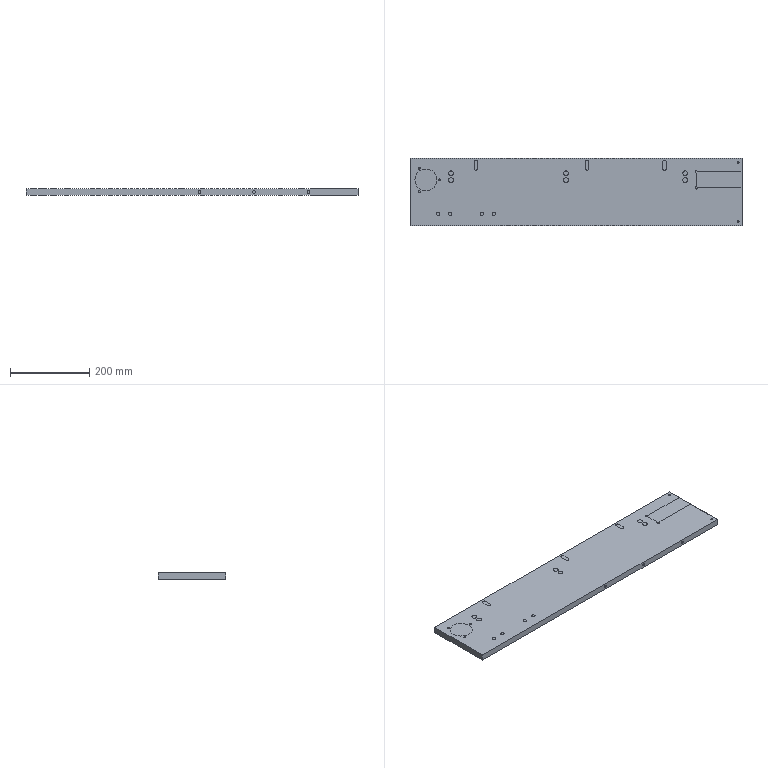NC program | NX | posted with a generic post | part box 836 x 170 x 16 mm
Lines 8598 to 9504 of 11551:
(等高清角 , TOOL : D4平底刀)
N17176 T16 M6
N17178 /M1
N17180 G17 G43 G0 G90 X721.292 Y95.484 Z100. S3000 H16 M3
N17182 Z0.1
N17184 G94 G1 Z-0.1 F800.
N17186 G3 X720.926 Y96.246 R0.45
N17188 X721.75 Y95.5 R-0.75 F1000.
N17190 G2 X721.97 Y96.47 R2.25
N17192 X721. Y96.25 R2.25
N17194 G1 X720.926 Y96.246
N17196 G3 X720.717 Y95.427 R0.45
N17198 G1 Z0.1
N17200 G0 Z0.
N17202 G1 Z-0.2 F800.
N17204 G2 X720.926 Y96.246 R0.45
N17206 G1 X721. Y96.25 F1000.
N17208 G3 X721.97 Y96.47 R2.25
N17210 X721.75 Y95.5 R2.25
N17212 G2 X720.926 Y96.246 R-0.75
N17214 X721.292 Y95.484 R0.45
N17216 G1 Z0.
N17218 G0 Z-0.1
N17220 G1 Z-0.3 F800.
N17222 G3 X720.926 Y96.246 R0.45
N17224 X721.75 Y95.5 R-0.75 F1000.
N17226 G2 X721.97 Y96.47 R2.25
N17228 X721. Y96.25 R2.25
N17230 G1 X720.926 Y96.246
N17232 G3 X720.717 Y95.427 R0.45
N17234 G1 Z-0.1
N17236 G0 Z-0.2
N17238 G1 Z-0.4 F800.
N17240 G2 X720.926 Y96.246 R0.45
N17242 G1 X721. Y96.25 F1000.
N17244 G3 X721.97 Y96.47 R2.25
N17246 X721.75 Y95.5 R2.25
N17248 G2 X720.926 Y96.246 R-0.75
N17250 X721.292 Y95.484 R0.45
N17252 G1 Z-0.2
N17254 G0 Z-0.3
N17256 G1 Z-0.5 F800.
N17258 G3 X720.926 Y96.246 R0.45
N17260 X721.75 Y95.5 R-0.75 F1000.
N17262 G2 X721.97 Y96.47 R2.25
N17264 X721. Y96.25 R2.25
N17266 G1 X720.926 Y96.246
N17268 G3 X720.717 Y95.427 R0.45
N17270 G1 Z-0.3
N17272 G0 Z-0.4
N17274 G1 Z-0.6 F800.
N17276 G2 X720.926 Y96.246 R0.45
N17278 G1 X721. Y96.25 F1000.
N17280 G3 X721.97 Y96.47 R2.25
N17282 X721.75 Y95.5 R2.25
N17284 G2 X720.926 Y96.246 R-0.75
N17286 X721.292 Y95.484 R0.45
N17288 G1 Z-0.4
N17290 G0 Z-0.5
N17292 G1 Z-0.7 F800.
N17294 G3 X720.926 Y96.246 R0.45
N17296 X721.75 Y95.5 R-0.75 F1000.
N17298 G2 X721.97 Y96.47 R2.25
N17300 X721. Y96.25 R2.25
N17302 G1 X720.926 Y96.246
N17304 G3 X720.717 Y95.427 R0.45
N17306 G1 Z-0.5
N17308 G0 Z-0.6
N17310 G1 Z-0.8 F800.
N17312 G2 X720.926 Y96.246 R0.45
N17314 G1 X721. Y96.25 F1000.
N17316 G3 X721.97 Y96.47 R2.25
N17318 X721.75 Y95.5 R2.25
N17320 G2 X720.926 Y96.246 R-0.75
N17322 X721.292 Y95.484 R0.45
N17324 G1 Z-0.6
N17326 G0 Z-0.7
N17328 G1 Z-0.9 F800.
N17330 G3 X720.926 Y96.246 R0.45
N17332 X721.75 Y95.5 R-0.75 F1000.
N17334 G2 X721.97 Y96.47 R2.25
N17336 X721. Y96.25 R2.25
N17338 G1 X720.926 Y96.246
N17340 G3 X720.717 Y95.427 R0.45
N17342 G1 Z-0.7
N17344 G0 Z-0.8
N17346 G1 Z-1. F800.
N17348 G2 X720.926 Y96.246 R0.45
N17350 G1 X721. Y96.25 F1000.
N17352 G3 X721.97 Y96.47 R2.25
N17354 X721.75 Y95.5 R2.25
N17356 G2 X720.926 Y96.246 R-0.75
N17358 X721.292 Y95.484 R0.45
N17360 G1 Z-0.8
N17362 G0 Z-0.9
N17364 G1 Z-1.1 F800.
N17366 G3 X720.926 Y96.246 R0.45
N17368 X721.75 Y95.5 R-0.75 F1000.
N17370 G2 X721.97 Y96.47 R2.25
N17372 X721. Y96.25 R2.25
N17374 G1 X720.926 Y96.246
N17376 G3 X720.717 Y95.427 R0.45
N17378 G1 Z-0.9
N17380 G0 Z-1.
N17382 G1 Z-1.2 F800.
N17384 G2 X720.926 Y96.246 R0.45
N17386 G1 X721. Y96.25 F1000.
N17388 G3 X721.97 Y96.47 R2.25
N17390 X721.75 Y95.5 R2.25
N17392 G2 X720.926 Y96.246 R-0.75
N17394 X721.292 Y95.484 R0.45
N17396 G1 Z-1.
N17398 G0 Z-1.1
N17400 G1 Z-1.3 F800.
N17402 G3 X720.926 Y96.246 R0.45
N17404 X721.75 Y95.5 R-0.75 F1000.
N17406 G2 X721.97 Y96.47 R2.25
N17408 X721. Y96.25 R2.25
N17410 G1 X720.926 Y96.246
N17412 G3 X720.717 Y95.427 R0.45
N17414 G1 Z-1.1
N17416 G0 Z-1.2
N17418 G1 Z-1.4 F800.
N17420 G2 X720.926 Y96.246 R0.45
N17422 G1 X721. Y96.25 F1000.
N17424 G3 X721.97 Y96.47 R2.25
N17426 X721.75 Y95.5 R2.25
N17428 G2 X720.926 Y96.246 R-0.75
N17430 X721.292 Y95.484 R0.45
N17432 G1 Z-1.2
N17434 G0 Z-1.3
N17436 G1 Z-1.5 F800.
N17438 G3 X720.926 Y96.246 R0.45
N17440 X721.75 Y95.5 R-0.75 F1000.
N17442 G2 X721.97 Y96.47 R2.25
N17444 X721. Y96.25 R2.25
N17446 G1 X720.926 Y96.246
N17448 G3 X720.717 Y95.427 R0.45
N17450 G1 Z-1.3
N17452 G0 Z-1.4
N17454 G1 Z-1.6 F800.
N17456 G2 X720.926 Y96.246 R0.45
N17458 G1 X721. Y96.25 F1000.
N17460 G3 X721.97 Y96.47 R2.25
N17462 X721.75 Y95.5 R2.25
N17464 G2 X720.926 Y96.246 R-0.75
N17466 X721.292 Y95.484 R0.45
N17468 G1 Z-1.4
N17470 G0 Z-1.5
N17472 G1 Z-1.7 F800.
N17474 G3 X720.926 Y96.246 R0.45
N17476 X721.75 Y95.5 R-0.75 F1000.
N17478 G2 X721.97 Y96.47 R2.25
N17480 X721. Y96.25 R2.25
N17482 G1 X720.926 Y96.246
N17484 G3 X720.717 Y95.427 R0.45
N17486 G1 Z-1.5
N17488 G0 Z-1.6
N17490 G1 Z-1.8 F800.
N17492 G2 X720.926 Y96.246 R0.45
N17494 G1 X721. Y96.25 F1000.
N17496 G3 X721.97 Y96.47 R2.25
N17498 X721.75 Y95.5 R2.25
N17500 G2 X720.926 Y96.246 R-0.75
N17502 X721.292 Y95.484 R0.45
N17504 G1 Z-1.6
N17506 G0 Z-1.7
N17508 G1 Z-1.9 F800.
N17510 G3 X720.926 Y96.246 R0.45
N17512 X721.75 Y95.5 R-0.75 F1000.
N17514 G2 X721.97 Y96.47 R2.25
N17516 X721. Y96.25 R2.25
N17518 G1 X720.926 Y96.246
N17520 G3 X720.717 Y95.427 R0.45
N17522 G1 Z-1.7
N17524 G0 Z-1.8
N17526 G1 Z-2. F800.
N17528 G2 X720.926 Y96.246 R0.45
N17530 G1 X721. Y96.25 F1000.
N17532 G3 X721.97 Y96.47 R2.25
N17534 X721.75 Y95.5 R2.25
N17536 G2 X720.926 Y96.246 R-0.75
N17538 X721.292 Y95.484 R0.45
N17540 G1 Z-1.8
N17542 G0 Z-1.9
N17544 G1 Z-2.1 F800.
N17546 G3 X720.926 Y96.246 R0.45
N17548 X721.75 Y95.5 R-0.75 F1000.
N17550 G2 X721.97 Y96.47 R2.25
N17552 X721. Y96.25 R2.25
N17554 G1 X720.926 Y96.246
N17556 G3 X720.717 Y95.427 R0.45
N17558 G1 Z-1.9
N17560 G0 Z-2.
N17562 G1 Z-2.2 F800.
N17564 G2 X720.926 Y96.246 R0.45
N17566 G1 X721. Y96.25 F1000.
N17568 G3 X721.97 Y96.47 R2.25
N17570 X721.75 Y95.5 R2.25
N17572 G2 X720.926 Y96.246 R-0.75
N17574 X721.292 Y95.484 R0.45
N17576 G1 Z-2.
N17578 G0 Z-2.1
N17580 G1 Z-2.3 F800.
N17582 G3 X720.926 Y96.246 R0.45
N17584 X721.75 Y95.5 R-0.75 F1000.
N17586 G2 X721.97 Y96.47 R2.25
N17588 X721. Y96.25 R2.25
N17590 G1 X720.926 Y96.246
N17592 G3 X720.717 Y95.427 R0.45
N17594 G1 Z-2.1
N17596 G0 Z-2.2
N17598 G1 Z-2.4 F800.
N17600 G2 X720.926 Y96.246 R0.45
N17602 G1 X721. Y96.25 F1000.
N17604 G3 X721.97 Y96.47 R2.25
N17606 X721.75 Y95.5 R2.25
N17608 G2 X720.926 Y96.246 R-0.75
N17610 X721.292 Y95.484 R0.45
N17612 G1 Z-2.2
N17614 G0 Z-2.3
N17616 G1 Z-2.5 F800.
N17618 G3 X720.926 Y96.246 R0.45
N17620 X721.75 Y95.5 R-0.75 F1000.
N17622 G2 X721.97 Y96.47 R2.25
N17624 X721. Y96.25 R2.25
N17626 G1 X720.926 Y96.246
N17628 G3 X720.717 Y95.427 R0.45
N17630 G1 Z-2.3
N17632 G0 Z-2.4
N17634 G1 Z-2.6 F800.
N17636 G2 X720.926 Y96.246 R0.45
N17638 G1 X721. Y96.25 F1000.
N17640 G3 X721.97 Y96.47 R2.25
N17642 X721.75 Y95.5 R2.25
N17644 G2 X720.926 Y96.246 R-0.75
N17646 X721.292 Y95.484 R0.45
N17648 G1 Z-2.4
N17650 G0 Z-2.5
N17652 G1 Z-2.7 F800.
N17654 G3 X720.926 Y96.246 R0.45
N17656 X721.75 Y95.5 R-0.75 F1000.
N17658 G2 X721.97 Y96.47 R2.25
N17660 X721. Y96.25 R2.25
N17662 G1 X720.926 Y96.246
N17664 G3 X720.717 Y95.427 R0.45
N17666 G1 Z-2.5
N17668 G0 Z-2.6
N17670 G1 Z-2.8 F800.
N17672 G2 X720.926 Y96.246 R0.45
N17674 G1 X721. Y96.25 F1000.
N17676 G3 X721.97 Y96.47 R2.25
N17678 X721.75 Y95.5 R2.25
N17680 G2 X720.926 Y96.246 R-0.75
N17682 X721.292 Y95.484 R0.45
N17684 G1 Z-2.6
N17686 G0 Z-2.7
N17688 G1 Z-2.9 F800.
N17690 G3 X720.926 Y96.246 R0.45
N17692 X721.75 Y95.5 R-0.75 F1000.
N17694 G2 X721.97 Y96.47 R2.25
N17696 X721. Y96.25 R2.25
N17698 G1 X720.926 Y96.246
N17700 G3 X720.717 Y95.427 R0.45
N17702 G1 Z-2.7
N17704 G0 Z-2.8
N17706 G1 Z-3. F800.
N17708 G2 X720.926 Y96.246 R0.45
N17710 G1 X721. Y96.25 F1000.
N17712 G3 X721.97 Y96.47 R2.25
N17714 X721.75 Y95.5 R2.25
N17716 G2 X720.926 Y96.246 R-0.75
N17718 X721.292 Y95.484 R0.45
N17720 G1 Z-2.8
N17722 G0 Z-2.9
N17724 G1 Z-3.1 F800.
N17726 G3 X720.926 Y96.246 R0.45
N17728 X721.75 Y95.5 R-0.75 F1000.
N17730 G2 X721.97 Y96.47 R2.25
N17732 X721. Y96.25 R2.25
N17734 G1 X720.926 Y96.246
N17736 G3 X720.717 Y95.427 R0.45
N17738 G1 Z-2.9
N17740 G0 Z-3.
N17742 G1 Z-3.2 F800.
N17744 G2 X720.926 Y96.246 R0.45
N17746 G1 X721. Y96.25 F1000.
N17748 G3 X721.97 Y96.47 R2.25
N17750 X721.75 Y95.5 R2.25
N17752 G2 X720.926 Y96.246 R-0.75
N17754 X721.292 Y95.484 R0.45
N17756 G1 Z-3.
N17758 G0 Z-3.1
N17760 G1 Z-3.3 F800.
N17762 G3 X720.926 Y96.246 R0.45
N17764 X721.75 Y95.5 R-0.75 F1000.
N17766 G2 X721.97 Y96.47 R2.25
N17768 X721. Y96.25 R2.25
N17770 G1 X720.926 Y96.246
N17772 G3 X720.717 Y95.427 R0.45
N17774 G1 Z-3.1
N17776 G0 Z-3.2
N17778 G1 Z-3.4 F800.
N17780 G2 X720.926 Y96.246 R0.45
N17782 G1 X721. Y96.25 F1000.
N17784 G3 X721.97 Y96.47 R2.25
N17786 X721.75 Y95.5 R2.25
N17788 G2 X720.926 Y96.246 R-0.75
N17790 X721.292 Y95.484 R0.45
N17792 G1 Z-3.2
N17794 G0 Z-3.3
N17796 G1 Z-3.5 F800.
N17798 G3 X720.926 Y96.246 R0.45
N17800 X721.75 Y95.5 R-0.75 F1000.
N17802 G2 X721.97 Y96.47 R2.25
N17804 X721. Y96.25 R2.25
N17806 G1 X720.926 Y96.246
N17808 G3 X720.717 Y95.427 R0.45
N17810 G1 Z-3.3
N17812 G0 Z-3.4
N17814 G1 Z-3.6 F800.
N17816 G2 X720.926 Y96.246 R0.45
N17818 G1 X721. Y96.25 F1000.
N17820 G3 X721.97 Y96.47 R2.25
N17822 X721.75 Y95.5 R2.25
N17824 G2 X720.926 Y96.246 R-0.75
N17826 X721.292 Y95.484 R0.45
N17828 G1 Z-3.4
N17830 G0 Z-3.5
N17832 G1 Z-3.7 F800.
N17834 G3 X720.926 Y96.246 R0.45
N17836 X721.75 Y95.5 R-0.75 F1000.
N17838 G2 X721.97 Y96.47 R2.25
N17840 X721. Y96.25 R2.25
N17842 G1 X720.926 Y96.246
N17844 G3 X720.717 Y95.427 R0.45
N17846 G1 Z-3.5
N17848 G0 Z-3.6
N17850 G1 Z-3.8 F800.
N17852 G2 X720.926 Y96.246 R0.45
N17854 G1 X721. Y96.25 F1000.
N17856 G3 X721.97 Y96.47 R2.25
N17858 X721.75 Y95.5 R2.25
N17860 G2 X720.926 Y96.246 R-0.75
N17862 X721.292 Y95.484 R0.45
N17864 G1 Z-3.6
N17866 G0 Z-3.7
N17868 G1 Z-3.9 F800.
N17870 G3 X720.926 Y96.246 R0.45
N17872 X721.75 Y95.5 R-0.75 F1000.
N17874 G2 X721.97 Y96.47 R2.25
N17876 X721. Y96.25 R2.25
N17878 G1 X720.926 Y96.246
N17880 G3 X720.717 Y95.427 R0.45
N17882 G1 Z-3.7
N17884 G0 Z-3.8
N17886 G1 Z-4. F800.
N17888 G2 X720.926 Y96.246 R0.45
N17890 G1 X721. Y96.25 F1000.
N17892 G3 X721.97 Y96.47 R2.25
N17894 X721.75 Y95.5 R2.25
N17896 G2 X720.926 Y96.246 R-0.75
N17898 X721.292 Y95.484 R0.45
N17900 G1 Z-3.8
N17902 G0 Z-3.9
N17904 G1 Z-4.1 F800.
N17906 G3 X720.926 Y96.246 R0.45
N17908 X721.75 Y95.5 R-0.75 F1000.
N17910 G2 X721.97 Y96.47 R2.25
N17912 X721. Y96.25 R2.25
N17914 G1 X720.926 Y96.246
N17916 G3 X720.717 Y95.427 R0.45
N17918 G1 Z-3.9
N17920 G0 Z-4.
N17922 G1 Z-4.2 F800.
N17924 G2 X720.926 Y96.246 R0.45
N17926 G1 X721. Y96.25 F1000.
N17928 G3 X721.97 Y96.47 R2.25
N17930 X721.75 Y95.5 R2.25
N17932 G2 X720.926 Y96.246 R-0.75
N17934 X721.292 Y95.484 R0.45
N17936 G1 Z-4.
N17938 G0 Z-4.1
N17940 G1 Z-4.3 F800.
N17942 G3 X720.926 Y96.246 R0.45
N17944 X721.75 Y95.5 R-0.75 F1000.
N17946 G2 X721.97 Y96.47 R2.25
N17948 X721. Y96.25 R2.25
N17950 G1 X720.926 Y96.246
N17952 G3 X720.717 Y95.427 R0.45
N17954 G1 Z-4.1
N17956 G0 Z-4.2
N17958 G1 Z-4.4 F800.
N17960 G2 X720.926 Y96.246 R0.45
N17962 G1 X721. Y96.25 F1000.
N17964 G3 X721.97 Y96.47 R2.25
N17966 X721.75 Y95.5 R2.25
N17968 G2 X720.926 Y96.246 R-0.75
N17970 X721.292 Y95.484 R0.45
N17972 G1 Z-4.2
N17974 G0 Z-4.3
N17976 G1 Z-4.5 F800.
N17978 G3 X720.926 Y96.246 R0.45
N17980 X721.75 Y95.5 R-0.75 F1000.
N17982 G2 X721.97 Y96.47 R2.25
N17984 X721. Y96.25 R2.25
N17986 G1 X720.926 Y96.246
N17988 G3 X720.717 Y95.427 R0.45
N17990 G1 Z-4.3
N17992 G0 Z-4.4
N17994 G1 Z-4.6 F800.
N17996 G2 X720.926 Y96.246 R0.45
N17998 G1 X721. Y96.25 F1000.
N18000 G3 X721.97 Y96.47 R2.25
N18002 X721.75 Y95.5 R2.25
N18004 G2 X720.926 Y96.246 R-0.75
N18006 X721.292 Y95.484 R0.45
N18008 G1 Z-4.4
N18010 G0 Z-4.5
N18012 G1 Z-4.7 F800.
N18014 G3 X720.926 Y96.246 R0.45
N18016 X721.75 Y95.5 R-0.75 F1000.
N18018 G2 X721.97 Y96.47 R2.25
N18020 X721. Y96.25 R2.25
N18022 G1 X720.926 Y96.246
N18024 G3 X720.717 Y95.427 R0.45
N18026 G1 Z-4.5
N18028 G0 Z-4.6
N18030 G1 Z-4.8 F800.
N18032 G2 X720.926 Y96.246 R0.45
N18034 G1 X721. Y96.25 F1000.
N18036 G3 X721.97 Y96.47 R2.25
N18038 X721.75 Y95.5 R2.25
N18040 G2 X720.926 Y96.246 R-0.75
N18042 X721.292 Y95.484 R0.45
N18044 G1 Z-4.6
N18046 G0 Z-4.7
N18048 G1 Z-4.9 F800.
N18050 G3 X720.926 Y96.246 R0.45
N18052 X721.75 Y95.5 R-0.75 F1000.
N18054 G2 X721.97 Y96.47 R2.25
N18056 X721. Y96.25 R2.25
N18058 G1 X720.926 Y96.246
N18060 G3 X720.717 Y95.427 R0.45
N18062 G1 Z-4.7
N18064 G0 Z-4.8
N18066 G1 Z-5. F800.
N18068 G2 X720.926 Y96.246 R0.45
N18070 G1 X721. Y96.25 F1000.
N18072 G3 X721.97 Y96.47 R2.25
N18074 X721.75 Y95.5 R2.25
N18076 G2 X720.926 Y96.246 R-0.75
N18078 X721.292 Y95.484 R0.45
N18080 G1 Z-4.8
N18082 G0 Z-4.9
N18084 G1 Z-5.1 F800.
N18086 G3 X720.926 Y96.246 R0.45
N18088 X721.75 Y95.5 R-0.75 F1000.
N18090 G2 X721.97 Y96.47 R2.25
N18092 X721. Y96.25 R2.25
N18094 G1 X720.926 Y96.246
N18096 G3 X720.717 Y95.427 R0.45
N18098 G1 Z-4.9
N18100 G0 Z-5.
N18102 G1 Z-5.2 F800.
N18104 G2 X720.926 Y96.246 R0.45
N18106 G1 X721. Y96.25 F1000.
N18108 G3 X721.97 Y96.47 R2.25
N18110 X721.75 Y95.5 R2.25
N18112 G2 X720.926 Y96.246 R-0.75
N18114 X721.292 Y95.484 R0.45
N18116 G1 Z-5.
N18118 G0 Z-5.1
N18120 G1 Z-5.3 F800.
N18122 G3 X720.926 Y96.246 R0.45
N18124 X721.75 Y95.5 R-0.75 F1000.
N18126 G2 X721.97 Y96.47 R2.25
N18128 X721. Y96.25 R2.25
N18130 G1 X720.926 Y96.246
N18132 G3 X720.717 Y95.427 R0.45
N18134 G1 Z-5.1
N18136 G0 Z-5.2
N18138 G1 Z-5.4 F800.
N18140 G2 X720.926 Y96.246 R0.45
N18142 G1 X721. Y96.25 F1000.
N18144 G3 X721.97 Y96.47 R2.25
N18146 X721.75 Y95.5 R2.25
N18148 G2 X720.926 Y96.246 R-0.75
N18150 X721.292 Y95.484 R0.45
N18152 G1 Z-5.2
N18154 G0 Z-5.3
N18156 G1 Z-5.5 F800.
N18158 G3 X720.926 Y96.246 R0.45
N18160 X721.75 Y95.5 R-0.75 F1000.
N18162 G2 X721.97 Y96.47 R2.25
N18164 X721. Y96.25 R2.25
N18166 G1 X720.926 Y96.246
N18168 G3 X720.717 Y95.427 R0.45
N18170 G1 Z-5.3
N18172 G0 Z-5.4
N18174 G1 Z-5.6 F800.
N18176 G2 X720.926 Y96.246 R0.45
N18178 G1 X721. Y96.25 F1000.
N18180 G3 X721.97 Y96.47 R2.25
N18182 X721.75 Y95.5 R2.25
N18184 G2 X720.926 Y96.246 R-0.75
N18186 X721.292 Y95.484 R0.45
N18188 G1 Z-5.4
N18190 G0 Z-5.5
N18192 G1 Z-5.7 F800.
N18194 G3 X720.926 Y96.246 R0.45
N18196 X721.75 Y95.5 R-0.75 F1000.
N18198 G2 X721.97 Y96.47 R2.25
N18200 X721. Y96.25 R2.25
N18202 G1 X720.926 Y96.246
N18204 G3 X720.717 Y95.427 R0.45
N18206 G1 Z-5.5
N18208 G0 Z-5.6
N18210 G1 Z-5.8 F800.
N18212 G2 X720.926 Y96.246 R0.45
N18214 G1 X721. Y96.25 F1000.
N18216 G3 X721.97 Y96.47 R2.25
N18218 X721.75 Y95.5 R2.25
N18220 G2 X720.926 Y96.246 R-0.75
N18222 X721.292 Y95.484 R0.45
N18224 G1 Z-5.6
N18226 G0 Z-5.7
N18228 G1 Z-5.9 F800.
N18230 G3 X720.926 Y96.246 R0.45
N18232 X721.75 Y95.5 R-0.75 F1000.
N18234 G2 X721.97 Y96.47 R2.25
N18236 X721. Y96.25 R2.25
N18238 G1 X720.926 Y96.246
N18240 G3 X720.717 Y95.427 R0.45
N18242 G1 Z-5.7
N18244 G0 Z-5.8
N18246 G1 Z-6. F800.
N18248 G2 X720.926 Y96.246 R0.45
N18250 G1 X721. Y96.25 F1000.
N18252 G3 X721.97 Y96.47 R2.25
N18254 X721.75 Y95.5 R2.25
N18256 G2 X720.926 Y96.246 R-0.75
N18258 X721.292 Y95.484 R0.45
N18260 G1 Z-5.8
N18262 G0 Z-5.9
N18264 G1 Z-6.1 F800.
N18266 G3 X720.926 Y96.246 R0.45
N18268 X721.75 Y95.5 R-0.75 F1000.
N18270 G2 X721.97 Y96.47 R2.25
N18272 X721. Y96.25 R2.25
N18274 G1 X720.926 Y96.246
N18276 G3 X720.717 Y95.427 R0.45
N18278 G1 Z-5.9
N18280 G0 Z-6.
N18282 G1 Z-6.2 F800.
N18284 G2 X720.926 Y96.246 R0.45
N18286 G1 X721. Y96.25 F1000.
N18288 G3 X721.97 Y96.47 R2.25
N18290 X721.75 Y95.5 R2.25
N18292 G2 X720.926 Y96.246 R-0.75
N18294 X721.292 Y95.484 R0.45
N18296 G1 Z-6.
N18298 G0 Z-6.1
N18300 G1 Z-6.3 F800.
N18302 G3 X720.926 Y96.246 R0.45
N18304 X721.75 Y95.5 R-0.75 F1000.
N18306 G2 X721.97 Y96.47 R2.25
N18308 X721. Y96.25 R2.25
N18310 G1 X720.926 Y96.246
N18312 G3 X720.717 Y95.427 R0.45
N18314 G1 Z-6.1
N18316 G0 Z-6.2
N18318 G1 Z-6.4 F800.
N18320 G2 X720.926 Y96.246 R0.45
N18322 G1 X721. Y96.25 F1000.
N18324 G3 X721.97 Y96.47 R2.25
N18326 X721.75 Y95.5 R2.25
N18328 G2 X720.926 Y96.246 R-0.75
N18330 X721.292 Y95.484 R0.45
N18332 G1 Z-6.2
N18334 G0 Z-6.3
N18336 G1 Z-6.5 F800.
N18338 G3 X720.926 Y96.246 R0.45
N18340 X721.75 Y95.5 R-0.75 F1000.
N18342 G2 X721.97 Y96.47 R2.25
N18344 X721. Y96.25 R2.25
N18346 G1 X720.926 Y96.246
N18348 G3 X720.717 Y95.427 R0.45
N18350 G1 Z-6.3
N18352 G0 Z-6.4
N18354 G1 Z-6.6 F800.
N18356 G2 X720.926 Y96.246 R0.45
N18358 G1 X721. Y96.25 F1000.
N18360 G3 X721.97 Y96.47 R2.25
N18362 X721.75 Y95.5 R2.25
N18364 G2 X720.926 Y96.246 R-0.75
N18366 X721.292 Y95.484 R0.45
N18368 G1 Z-6.4
N18370 G0 Z-6.5
N18372 G1 Z-6.7 F800.
N18374 G3 X720.926 Y96.246 R0.45
N18376 X721.75 Y95.5 R-0.75 F1000.
N18378 G2 X721.97 Y96.47 R2.25
N18380 X721. Y96.25 R2.25
N18382 G1 X720.926 Y96.246
N18384 G3 X720.717 Y95.427 R0.45
N18386 G1 Z-6.5
N18388 G0 Z-6.6
N18390 G1 Z-6.8 F800.
N18392 G2 X720.926 Y96.246 R0.45
N18394 G1 X721. Y96.25 F1000.
N18396 G3 X721.97 Y96.47 R2.25
N18398 X721.75 Y95.5 R2.25
N18400 G2 X720.926 Y96.246 R-0.75
N18402 X721.292 Y95.484 R0.45
N18404 G1 Z-6.6
N18406 G0 Z-6.7
N18408 G1 Z-6.9 F800.
N18410 G3 X720.926 Y96.246 R0.45
N18412 X721.75 Y95.5 R-0.75 F1000.
N18414 G2 X721.97 Y96.47 R2.25
N18416 X721. Y96.25 R2.25
N18418 G1 X720.926 Y96.246
N18420 G3 X720.717 Y95.427 R0.45
N18422 G1 Z-6.7
N18424 G0 Z-6.8
N18426 G1 Z-7. F800.
N18428 G2 X720.926 Y96.246 R0.45
N18430 G1 X721. Y96.25 F1000.
N18432 G3 X721.97 Y96.47 R2.25
N18434 X721.75 Y95.5 R2.25
N18436 G2 X720.926 Y96.246 R-0.75
N18438 X721.292 Y95.484 R0.45
N18440 G1 Z-6.8
N18442 G0 Z-6.9
N18444 G1 Z-7.1 F800.
N18446 G3 X720.926 Y96.246 R0.45
N18448 X721.75 Y95.5 R-0.75 F1000.
N18450 G2 X721.97 Y96.47 R2.25
N18452 X721. Y96.25 R2.25
N18454 G1 X720.926 Y96.246
N18456 G3 X720.717 Y95.427 R0.45
N18458 G1 Z-6.9
N18460 G0 Z-7.
N18462 G1 Z-7.2 F800.
N18464 G2 X720.926 Y96.246 R0.45
N18466 G1 X721. Y96.25 F1000.
N18468 G3 X721.97 Y96.47 R2.25
N18470 X721.75 Y95.5 R2.25
N18472 G2 X720.926 Y96.246 R-0.75
N18474 X721.292 Y95.484 R0.45
N18476 G1 Z-7.
N18478 G0 Z-7.1
N18480 G1 Z-7.3 F800.
N18482 G3 X720.926 Y96.246 R0.45
N18484 X721.75 Y95.5 R-0.75 F1000.
N18486 G2 X721.97 Y96.47 R2.25
N18488 X721. Y96.25 R2.25
N18490 G1 X720.926 Y96.246
N18492 G3 X720.717 Y95.427 R0.45
N18494 G1 Z-7.1
N18496 G0 Z-7.2
N18498 G1 Z-7.4 F800.
N18500 G2 X720.926 Y96.246 R0.45
N18502 G1 X721. Y96.25 F1000.
N18504 G3 X721.97 Y96.47 R2.25
N18506 X721.75 Y95.5 R2.25
N18508 G2 X720.926 Y96.246 R-0.75
N18510 X721.292 Y95.484 R0.45
N18512 G1 Z-7.2
N18514 G0 Z-7.3
N18516 G1 Z-7.5 F800.
N18518 G3 X720.926 Y96.246 R0.45
N18520 X721.75 Y95.5 R-0.75 F1000.
N18522 G2 X721.97 Y96.47 R2.25
N18524 X721. Y96.25 R2.25
N18526 G1 X720.926 Y96.246
N18528 G3 X720.717 Y95.427 R0.45
N18530 G1 Z-7.3
N18532 G0 Z-7.4
N18534 G1 Z-7.6 F800.
N18536 G2 X720.926 Y96.246 R0.45
N18538 G1 X721. Y96.25 F1000.
N18540 G3 X721.97 Y96.47 R2.25
N18542 X721.75 Y95.5 R2.25
N18544 G2 X720.926 Y96.246 R-0.75
N18546 X721.292 Y95.484 R0.45
N18548 G1 Z-7.4
N18550 G0 Z-7.5
N18552 G1 Z-7.7 F800.
N18554 G3 X720.926 Y96.246 R0.45
N18556 X721.75 Y95.5 R-0.75 F1000.
N18558 G2 X721.97 Y96.47 R2.25
N18560 X721. Y96.25 R2.25
N18562 G1 X720.926 Y96.246
N18564 G3 X720.717 Y95.427 R0.45
N18566 G1 Z-7.5
N18568 G0 Z-7.6
N18570 G1 Z-7.8 F800.
N18572 G2 X720.926 Y96.246 R0.45
N18574 G1 X721. Y96.25 F1000.
N18576 G3 X721.97 Y96.47 R2.25
N18578 X721.75 Y95.5 R2.25
N18580 G2 X720.926 Y96.246 R-0.75
N18582 X721.292 Y95.484 R0.45
N18584 G1 Z-7.6
N18586 G0 Z-7.7
N18588 G1 Z-7.9 F800.
N18590 G3 X720.926 Y96.246 R0.45
N18592 X721.75 Y95.5 R-0.75 F1000.
N18594 G2 X721.97 Y96.47 R2.25
N18596 X721. Y96.25 R2.25
N18598 G1 X720.926 Y96.246
N18600 G3 X720.717 Y95.427 R0.45
N18602 G1 Z-7.7
N18604 G0 Z-7.8
N18606 G1 Z-8. F800.
N18608 G2 X720.926 Y96.246 R0.45
N18610 G1 X721. Y96.25 F1000.
N18612 G3 X721.97 Y96.47 R2.25
N18614 X721.75 Y95.5 R2.25
N18616 G2 X720.926 Y96.246 R-0.75
N18618 X721.292 Y95.484 R0.45
N18620 G1 Z-7.8
N18622 G0 Z-7.9
N18624 G1 Z-8.1 F800.
N18626 G3 X720.926 Y96.246 R0.45
N18628 X721.75 Y95.5 R-0.75 F1000.
N18630 G2 X721.97 Y96.47 R2.25
N18632 X721. Y96.25 R2.25
N18634 G1 X720.926 Y96.246
N18636 G3 X720.717 Y95.427 R0.45
N18638 G1 Z-7.9
N18640 G0 Z-8.
N18642 G1 Z-8.2 F800.
N18644 G2 X720.926 Y96.246 R0.45
N18646 G1 X721. Y96.25 F1000.
N18648 G3 X721.97 Y96.47 R2.25
N18650 X721.75 Y95.5 R2.25
N18652 G2 X720.926 Y96.246 R-0.75
N18654 X721.292 Y95.484 R0.45
N18656 G1 Z-8.
N18658 G0 Z-8.1
N18660 G1 Z-8.3 F800.
N18662 G3 X720.926 Y96.246 R0.45
N18664 X721.75 Y95.5 R-0.75 F1000.
N18666 G2 X721.97 Y96.47 R2.25
N18668 X721. Y96.25 R2.25
N18670 G1 X720.926 Y96.246
N18672 G3 X720.717 Y95.427 R0.45
N18674 G1 Z-8.1
N18676 G0 Z-8.2
N18678 G1 Z-8.4 F800.
N18680 G2 X720.926 Y96.246 R0.45
N18682 G1 X721. Y96.25 F1000.
N18684 G3 X721.97 Y96.47 R2.25
N18686 X721.75 Y95.5 R2.25
N18688 G2 X720.926 Y96.246 R-0.75
N18690 X721.292 Y95.484 R0.45
N18692 G1 Z-8.2
N18694 G0 Z-8.3
N18696 G1 Z-8.5 F800.
N18698 G3 X720.926 Y96.246 R0.45
N18700 X721.75 Y95.5 R-0.75 F1000.
N18702 G2 X721.97 Y96.47 R2.25
N18704 X721. Y96.25 R2.25
N18706 G1 X720.926 Y96.246
N18708 G3 X720.717 Y95.427 R0.45
N18710 G1 Z-8.3
N18712 G0 Z-8.4
N18714 G1 Z-8.6 F800.
N18716 G2 X720.926 Y96.246 R0.45
N18718 G1 X721. Y96.25 F1000.
N18720 G3 X721.97 Y96.47 R2.25
N18722 X721.75 Y95.5 R2.25
N18724 G2 X720.926 Y96.246 R-0.75
N18726 X721.292 Y95.484 R0.45
N18728 G1 Z-8.4
N18730 G0 Z-8.5
N18732 G1 Z-8.7 F800.
N18734 G3 X720.926 Y96.246 R0.45
N18736 X721.75 Y95.5 R-0.75 F1000.
N18738 G2 X721.97 Y96.47 R2.25
N18740 X721. Y96.25 R2.25
N18742 G1 X720.926 Y96.246
N18744 G3 X720.717 Y95.427 R0.45
N18746 G1 Z-8.5
N18748 G0 Z-8.6
N18750 G1 Z-8.8 F800.
N18752 G2 X720.926 Y96.246 R0.45
N18754 G1 X721. Y96.25 F1000.
N18756 G3 X721.97 Y96.47 R2.25
N18758 X721.75 Y95.5 R2.25
N18760 G2 X720.926 Y96.246 R-0.75
N18762 X721.292 Y95.484 R0.45
N18764 G1 Z-8.6
N18766 G0 Z-8.7
N18768 G1 Z-8.9 F800.
N18770 G3 X720.926 Y96.246 R0.45
N18772 X721.75 Y95.5 R-0.75 F1000.
N18774 G2 X721.97 Y96.47 R2.25
N18776 X721. Y96.25 R2.25
N18778 G1 X720.926 Y96.246
N18780 G3 X720.717 Y95.427 R0.45
N18782 G1 Z-8.7
N18784 G0 Z-8.8
N18786 G1 Z-9. F800.
N18788 G2 X720.926 Y96.246 R0.45
N18790 G1 X721. Y96.25 F1000.
N18792 G3 X721.97 Y96.47 R2.25
N18794 X721.75 Y95.5 R2.25
N18796 G2 X720.926 Y96.246 R-0.75
N18798 X721.292 Y95.484 R0.45
N18800 G1 Z-8.8
N18802 G0 Z-8.9
N18804 G1 Z-9.1 F800.
N18806 G3 X720.926 Y96.246 R0.45
N18808 X721.75 Y95.5 R-0.75 F1000.
N18810 G2 X721.97 Y96.47 R2.25
N18812 X721. Y96.25 R2.25
N18814 G1 X720.926 Y96.246
N18816 G3 X720.717 Y95.427 R0.45
N18818 G1 Z-8.9
N18820 G0 Z-9.
N18822 G1 Z-9.2 F800.
N18824 G2 X720.926 Y96.246 R0.45
N18826 G1 X721. Y96.25 F1000.
N18828 G3 X721.97 Y96.47 R2.25
N18830 X721.75 Y95.5 R2.25
N18832 G2 X720.926 Y96.246 R-0.75
N18834 X721.292 Y95.484 R0.45
N18836 G1 Z-9.
N18838 G0 Z-9.1
N18840 G1 Z-9.3 F800.
N18842 G3 X720.926 Y96.246 R0.45
N18844 X721.75 Y95.5 R-0.75 F1000.
N18846 G2 X721.97 Y96.47 R2.25
N18848 X721. Y96.25 R2.25
N18850 G1 X720.926 Y96.246
N18852 G3 X720.717 Y95.427 R0.45
N18854 G1 Z-9.1
N18856 G0 Z-9.2
N18858 G1 Z-9.4 F800.
N18860 G2 X720.926 Y96.246 R0.45
N18862 G1 X721. Y96.25 F1000.
N18864 G3 X721.97 Y96.47 R2.25
N18866 X721.75 Y95.5 R2.25
N18868 G2 X720.926 Y96.246 R-0.75
N18870 X721.292 Y95.484 R0.45
N18872 G1 Z-9.2
N18874 G0 Z-9.3
N18876 G1 Z-9.5 F800.
N18878 G3 X720.926 Y96.246 R0.45
N18880 X721.75 Y95.5 R-0.75 F1000.
N18882 G2 X721.97 Y96.47 R2.25
N18884 X721. Y96.25 R2.25
N18886 G1 X720.926 Y96.246
N18888 G3 X720.717 Y95.427 R0.45
N18890 G1 Z-9.3
N18892 G0 Z-9.4
N18894 G1 Z-9.6 F800.
N18896 G2 X720.926 Y96.246 R0.45
N18898 G1 X721. Y96.25 F1000.
N18900 G3 X721.97 Y96.47 R2.25
N18902 X721.75 Y95.5 R2.25
N18904 G2 X720.926 Y96.246 R-0.75
N18906 X721.292 Y95.484 R0.45
N18908 G1 Z-9.4
N18910 G0 Z-9.5
N18912 G1 Z-9.7 F800.
N18914 G3 X720.926 Y96.246 R0.45
N18916 X721.75 Y95.5 R-0.75 F1000.
N18918 G2 X721.97 Y96.47 R2.25
N18920 X721. Y96.25 R2.25
N18922 G1 X720.926 Y96.246
N18924 G3 X720.717 Y95.427 R0.45
N18926 G1 Z-9.5
N18928 G0 Z-9.6
N18930 G1 Z-9.8 F800.
N18932 G2 X720.926 Y96.246 R0.45
N18934 G1 X721. Y96.25 F1000.
N18936 G3 X721.97 Y96.47 R2.25
N18938 X721.75 Y95.5 R2.25
N18940 G2 X720.926 Y96.246 R-0.75
N18942 X721.292 Y95.484 R0.45
N18944 G1 Z-9.6
N18946 G0 Z-9.7
N18948 G1 Z-9.9 F800.
N18950 G3 X720.926 Y96.246 R0.45
N18952 X721.75 Y95.5 R-0.75 F1000.
N18954 G2 X721.97 Y96.47 R2.25
N18956 X721. Y96.25 R2.25
N18958 G1 X720.926 Y96.246
N18960 G3 X720.717 Y95.427 R0.45
N18962 G1 Z-9.7
N18964 G0 Z-9.8
N18966 G1 Z-10. F800.
N18968 G2 X720.926 Y96.246 R0.45
N18970 G1 X721. Y96.25 F1000.
N18972 G3 X721.97 Y96.47 R2.25
N18974 X721.75 Y95.5 R2.25
N18976 G2 X720.926 Y96.246 R-0.75
N18978 X721.292 Y95.484 R0.45
N18980 G1 Z-9.8
N18982 G0 Z-9.9